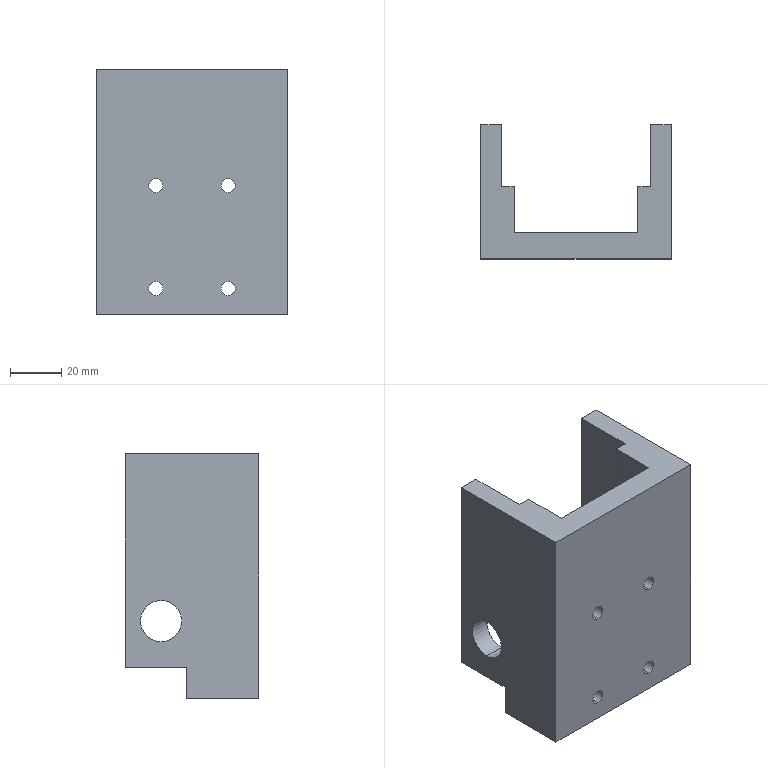Part | SolidWorks | features ICE 6, Extrusion 1 | 1 solid | 52 faces | box 74 x 52 x 95 mm | volume 141105 mm3 | cylinder 28 | plane 24 | commonest cylinder face diameters 5.5 x8 10 x8 2.5 x4 3 x4 16 x4
STEP:
#1=CARTESIAN_POINT('',(31.034,10.,22.));
#2=VERTEX_POINT('',#1);
#3=CARTESIAN_POINT('',(31.034,10.,38.));
#4=VERTEX_POINT('',#3);
#5=CARTESIAN_POINT('',(31.034,10.,30.));
#6=DIRECTION('',(-1.,0.,0.));
#7=DIRECTION('',(0.,0.,1.));
#8=AXIS2_PLACEMENT_3D('',#5,#6,#7);
#9=CIRCLE('',#8,8.);
#10=EDGE_CURVE('',#2,#4,#9,.T.);
#11=ORIENTED_EDGE('',*,*,#10,.F.);
#12=CARTESIAN_POINT('',(23.034,10.,22.));
#13=VERTEX_POINT('',#12);
#14=CARTESIAN_POINT('',(31.034,10.,22.));
#15=DIRECTION('',(-1.,0.,0.));
#16=VECTOR('',#15,1000.);
#17=LINE('',#14,#16);
#18=EDGE_CURVE('',#2,#13,#17,.T.);
#19=ORIENTED_EDGE('',*,*,#18,.T.);
#20=CARTESIAN_POINT('',(23.034,10.,38.));
#21=VERTEX_POINT('',#20);
#22=CARTESIAN_POINT('',(23.034,10.,30.));
#23=DIRECTION('',(1.,0.,0.));
#24=DIRECTION('',(0.,1.,0.));
#25=AXIS2_PLACEMENT_3D('',#22,#23,#24);
#26=CIRCLE('',#25,8.);
#27=EDGE_CURVE('',#21,#13,#26,.T.);
#28=ORIENTED_EDGE('',*,*,#27,.F.);
#29=CARTESIAN_POINT('',(31.034,10.,38.));
#30=DIRECTION('',(-1.,0.,0.));
#31=VECTOR('',#30,1000.);
#32=LINE('',#29,#31);
#33=EDGE_CURVE('',#4,#21,#32,.T.);
#34=ORIENTED_EDGE('',*,*,#33,.F.);
#35=EDGE_LOOP('',(#11,#19,#28,#34));
#36=FACE_OUTER_BOUND('',#35,.T.);
#37=CARTESIAN_POINT('',(31.034,10.,30.));
#38=DIRECTION('',(-1.,0.,0.));
#39=DIRECTION('',(0.,0.,1.));
#40=AXIS2_PLACEMENT_3D('',#37,#38,#39);
#41=CYLINDRICAL_SURFACE('',#40,8.);
#42=ADVANCED_FACE('',(#36),#41,.F.);
#43=CARTESIAN_POINT('',(-34.966,10.,22.));
#44=VERTEX_POINT('',#43);
#45=CARTESIAN_POINT('',(-34.966,10.,38.));
#46=VERTEX_POINT('',#45);
#47=CARTESIAN_POINT('',(-34.966,10.,30.));
#48=DIRECTION('',(-1.,0.,0.));
#49=DIRECTION('',(0.,0.,1.));
#50=AXIS2_PLACEMENT_3D('',#47,#48,#49);
#51=CIRCLE('',#50,8.);
#52=EDGE_CURVE('',#44,#46,#51,.T.);
#53=ORIENTED_EDGE('',*,*,#52,.F.);
#54=CARTESIAN_POINT('',(-42.966,10.,22.));
#55=VERTEX_POINT('',#54);
#56=CARTESIAN_POINT('',(31.034,10.,22.));
#57=DIRECTION('',(-1.,0.,0.));
#58=VECTOR('',#57,1000.);
#59=LINE('',#56,#58);
#60=EDGE_CURVE('',#44,#55,#59,.T.);
#61=ORIENTED_EDGE('',*,*,#60,.T.);
#62=CARTESIAN_POINT('',(-42.966,10.,38.));
#63=VERTEX_POINT('',#62);
#64=CARTESIAN_POINT('',(-42.966,10.,30.));
#65=DIRECTION('',(-1.,0.,0.));
#66=DIRECTION('',(0.,0.,1.));
#67=AXIS2_PLACEMENT_3D('',#64,#65,#66);
#68=CIRCLE('',#67,8.);
#69=EDGE_CURVE('',#55,#63,#68,.T.);
#70=ORIENTED_EDGE('',*,*,#69,.T.);
#71=CARTESIAN_POINT('',(31.034,10.,38.));
#72=DIRECTION('',(-1.,0.,0.));
#73=VECTOR('',#72,1000.);
#74=LINE('',#71,#73);
#75=EDGE_CURVE('',#46,#63,#74,.T.);
#76=ORIENTED_EDGE('',*,*,#75,.F.);
#77=EDGE_LOOP('',(#53,#61,#70,#76));
#78=FACE_OUTER_BOUND('',#77,.T.);
#79=CARTESIAN_POINT('',(31.034,10.,30.));
#80=DIRECTION('',(-1.,0.,0.));
#81=DIRECTION('',(0.,0.,1.));
#82=AXIS2_PLACEMENT_3D('',#79,#80,#81);
#83=CYLINDRICAL_SURFACE('',#82,8.);
#84=ADVANCED_FACE('',(#78),#83,.F.);
#85=CARTESIAN_POINT('',(-32.466,-7.5,8.75));
#86=VERTEX_POINT('',#85);
#87=CARTESIAN_POINT('',(-32.466,-7.5,11.25));
#88=VERTEX_POINT('',#87);
#89=CARTESIAN_POINT('',(-32.466,-7.5,10.));
#90=DIRECTION('',(0.,1.,0.));
#91=DIRECTION('',(0.,0.,1.));
#92=AXIS2_PLACEMENT_3D('',#89,#90,#91);
#93=CIRCLE('',#92,1.25);
#94=EDGE_CURVE('',#86,#88,#93,.T.);
#95=ORIENTED_EDGE('',*,*,#94,.F.);
#96=CARTESIAN_POINT('',(-32.466,-6.,8.75));
#97=VERTEX_POINT('',#96);
#98=CARTESIAN_POINT('',(-32.466,-7.5,8.75));
#99=DIRECTION('',(0.,1.,0.));
#100=VECTOR('',#99,1000.);
#101=LINE('',#98,#100);
#102=EDGE_CURVE('',#86,#97,#101,.T.);
#103=ORIENTED_EDGE('',*,*,#102,.T.);
#104=CARTESIAN_POINT('',(-32.466,-6.,11.25));
#105=VERTEX_POINT('',#104);
#106=CARTESIAN_POINT('',(-32.466,-6.,10.));
#107=DIRECTION('',(0.,-1.,0.));
#108=DIRECTION('',(0.,0.,1.));
#109=AXIS2_PLACEMENT_3D('',#106,#107,#108);
#110=CIRCLE('',#109,1.25);
#111=EDGE_CURVE('',#105,#97,#110,.T.);
#112=ORIENTED_EDGE('',*,*,#111,.F.);
#113=CARTESIAN_POINT('',(-32.466,-7.5,11.25));
#114=DIRECTION('',(0.,1.,0.));
#115=VECTOR('',#114,1000.);
#116=LINE('',#113,#115);
#117=EDGE_CURVE('',#88,#105,#116,.T.);
#118=ORIENTED_EDGE('',*,*,#117,.F.);
#119=EDGE_LOOP('',(#95,#103,#112,#118));
#120=FACE_OUTER_BOUND('',#119,.T.);
#121=CARTESIAN_POINT('',(-32.466,-7.5,10.));
#122=DIRECTION('',(0.,1.,0.));
#123=DIRECTION('',(0.,0.,1.));
#124=AXIS2_PLACEMENT_3D('',#121,#122,#123);
#125=CYLINDRICAL_SURFACE('',#124,1.25);
#126=ADVANCED_FACE('',(#120),#125,.F.);
#127=CARTESIAN_POINT('',(20.534,-7.5,8.75));
#128=VERTEX_POINT('',#127);
#129=CARTESIAN_POINT('',(20.534,-7.5,11.25));
#130=VERTEX_POINT('',#129);
#131=CARTESIAN_POINT('',(20.534,-7.5,10.));
#132=DIRECTION('',(0.,1.,0.));
#133=DIRECTION('',(0.,0.,1.));
#134=AXIS2_PLACEMENT_3D('',#131,#132,#133);
#135=CIRCLE('',#134,1.25);
#136=EDGE_CURVE('',#128,#130,#135,.T.);
#137=ORIENTED_EDGE('',*,*,#136,.F.);
#138=CARTESIAN_POINT('',(20.534,-6.,8.75));
#139=VERTEX_POINT('',#138);
#140=CARTESIAN_POINT('',(20.534,-7.5,8.75));
#141=DIRECTION('',(0.,1.,0.));
#142=VECTOR('',#141,1000.);
#143=LINE('',#140,#142);
#144=EDGE_CURVE('',#128,#139,#143,.T.);
#145=ORIENTED_EDGE('',*,*,#144,.T.);
#146=CARTESIAN_POINT('',(20.534,-6.,11.25));
#147=VERTEX_POINT('',#146);
#148=CARTESIAN_POINT('',(20.534,-6.,10.));
#149=DIRECTION('',(0.,-1.,0.));
#150=DIRECTION('',(0.,0.,1.));
#151=AXIS2_PLACEMENT_3D('',#148,#149,#150);
#152=CIRCLE('',#151,1.25);
#153=EDGE_CURVE('',#147,#139,#152,.T.);
#154=ORIENTED_EDGE('',*,*,#153,.F.);
#155=CARTESIAN_POINT('',(20.534,-7.5,11.25));
#156=DIRECTION('',(0.,1.,0.));
#157=VECTOR('',#156,1000.);
#158=LINE('',#155,#157);
#159=EDGE_CURVE('',#130,#147,#158,.T.);
#160=ORIENTED_EDGE('',*,*,#159,.F.);
#161=EDGE_LOOP('',(#137,#145,#154,#160));
#162=FACE_OUTER_BOUND('',#161,.T.);
#163=CARTESIAN_POINT('',(20.534,-7.5,10.));
#164=DIRECTION('',(0.,1.,0.));
#165=DIRECTION('',(0.,0.,1.));
#166=AXIS2_PLACEMENT_3D('',#163,#164,#165);
#167=CYLINDRICAL_SURFACE('',#166,1.25);
#168=ADVANCED_FACE('',(#162),#167,.F.);
#169=CARTESIAN_POINT('',(-32.466,-6.,8.5));
#170=VERTEX_POINT('',#169);
#171=CARTESIAN_POINT('',(-32.466,-6.,11.5));
#172=VERTEX_POINT('',#171);
#173=CARTESIAN_POINT('',(-32.466,-6.,10.));
#174=DIRECTION('',(0.,1.,0.));
#175=DIRECTION('',(0.,0.,1.));
#176=AXIS2_PLACEMENT_3D('',#173,#174,#175);
#177=CIRCLE('',#176,1.5);
#178=EDGE_CURVE('',#170,#172,#177,.T.);
#179=ORIENTED_EDGE('',*,*,#178,.F.);
#180=CARTESIAN_POINT('',(-32.466,0.,8.5));
#181=VERTEX_POINT('',#180);
#182=CARTESIAN_POINT('',(-32.466,-6.,8.5));
#183=DIRECTION('',(0.,1.,0.));
#184=VECTOR('',#183,1000.);
#185=LINE('',#182,#184);
#186=EDGE_CURVE('',#170,#181,#185,.T.);
#187=ORIENTED_EDGE('',*,*,#186,.T.);
#188=CARTESIAN_POINT('',(-32.466,0.,11.5));
#189=VERTEX_POINT('',#188);
#190=CARTESIAN_POINT('',(-32.466,0.,10.));
#191=DIRECTION('',(0.,1.,0.));
#192=DIRECTION('',(0.,0.,1.));
#193=AXIS2_PLACEMENT_3D('',#190,#191,#192);
#194=CIRCLE('',#193,1.5);
#195=EDGE_CURVE('',#181,#189,#194,.T.);
#196=ORIENTED_EDGE('',*,*,#195,.T.);
#197=CARTESIAN_POINT('',(-32.466,-6.,11.5));
#198=DIRECTION('',(0.,1.,0.));
#199=VECTOR('',#198,1000.);
#200=LINE('',#197,#199);
#201=EDGE_CURVE('',#172,#189,#200,.T.);
#202=ORIENTED_EDGE('',*,*,#201,.F.);
#203=EDGE_LOOP('',(#179,#187,#196,#202));
#204=FACE_OUTER_BOUND('',#203,.T.);
#205=CARTESIAN_POINT('',(-32.466,-6.,10.));
#206=DIRECTION('',(0.,1.,0.));
#207=DIRECTION('',(0.,0.,1.));
#208=AXIS2_PLACEMENT_3D('',#205,#206,#207);
#209=CYLINDRICAL_SURFACE('',#208,1.5);
#210=ADVANCED_FACE('',(#204),#209,.F.);
#211=CARTESIAN_POINT('',(20.534,-6.,8.5));
#212=VERTEX_POINT('',#211);
#213=CARTESIAN_POINT('',(20.534,-6.,11.5));
#214=VERTEX_POINT('',#213);
#215=CARTESIAN_POINT('',(20.534,-6.,10.));
#216=DIRECTION('',(0.,1.,0.));
#217=DIRECTION('',(0.,0.,1.));
#218=AXIS2_PLACEMENT_3D('',#215,#216,#217);
#219=CIRCLE('',#218,1.5);
#220=EDGE_CURVE('',#212,#214,#219,.T.);
#221=ORIENTED_EDGE('',*,*,#220,.F.);
#222=CARTESIAN_POINT('',(20.534,0.,8.5));
#223=VERTEX_POINT('',#222);
#224=CARTESIAN_POINT('',(20.534,-6.,8.5));
#225=DIRECTION('',(0.,1.,0.));
#226=VECTOR('',#225,1000.);
#227=LINE('',#224,#226);
#228=EDGE_CURVE('',#212,#223,#227,.T.);
#229=ORIENTED_EDGE('',*,*,#228,.T.);
#230=CARTESIAN_POINT('',(20.534,0.,11.5));
#231=VERTEX_POINT('',#230);
#232=CARTESIAN_POINT('',(20.534,0.,10.));
#233=DIRECTION('',(0.,1.,0.));
#234=DIRECTION('',(0.,0.,1.));
#235=AXIS2_PLACEMENT_3D('',#232,#233,#234);
#236=CIRCLE('',#235,1.5);
#237=EDGE_CURVE('',#223,#231,#236,.T.);
#238=ORIENTED_EDGE('',*,*,#237,.T.);
#239=CARTESIAN_POINT('',(20.534,-6.,11.5));
#240=DIRECTION('',(0.,1.,0.));
#241=VECTOR('',#240,1000.);
#242=LINE('',#239,#241);
#243=EDGE_CURVE('',#214,#231,#242,.T.);
#244=ORIENTED_EDGE('',*,*,#243,.F.);
#245=EDGE_LOOP('',(#221,#229,#238,#244));
#246=FACE_OUTER_BOUND('',#245,.T.);
#247=CARTESIAN_POINT('',(20.534,-6.,10.));
#248=DIRECTION('',(0.,1.,0.));
#249=DIRECTION('',(0.,0.,1.));
#250=AXIS2_PLACEMENT_3D('',#247,#248,#249);
#251=CYLINDRICAL_SURFACE('',#250,1.5);
#252=ADVANCED_FACE('',(#246),#251,.F.);
#253=CARTESIAN_POINT('',(-19.966,-23.75,5.));
#254=VERTEX_POINT('',#253);
#255=CARTESIAN_POINT('',(-19.966,-23.75,15.));
#256=VERTEX_POINT('',#255);
#257=CARTESIAN_POINT('',(-19.966,-23.75,10.));
#258=DIRECTION('',(0.,1.,0.));
#259=DIRECTION('',(0.,0.,1.));
#260=AXIS2_PLACEMENT_3D('',#257,#258,#259);
#261=CIRCLE('',#260,5.);
#262=EDGE_CURVE('',#254,#256,#261,.T.);
#263=ORIENTED_EDGE('',*,*,#262,.F.);
#264=CARTESIAN_POINT('',(-19.966,-18.,5.));
#265=VERTEX_POINT('',#264);
#266=CARTESIAN_POINT('',(-19.966,-23.75,5.));
#267=DIRECTION('',(0.,1.,0.));
#268=VECTOR('',#267,1000.);
#269=LINE('',#266,#268);
#270=EDGE_CURVE('',#254,#265,#269,.T.);
#271=ORIENTED_EDGE('',*,*,#270,.T.);
#272=CARTESIAN_POINT('',(-19.966,-18.,15.));
#273=VERTEX_POINT('',#272);
#274=CARTESIAN_POINT('',(-19.966,-18.,10.));
#275=DIRECTION('',(0.,1.,0.));
#276=DIRECTION('',(0.,0.,1.));
#277=AXIS2_PLACEMENT_3D('',#274,#275,#276);
#278=CIRCLE('',#277,5.);
#279=EDGE_CURVE('',#265,#273,#278,.T.);
#280=ORIENTED_EDGE('',*,*,#279,.T.);
#281=CARTESIAN_POINT('',(-19.966,-23.75,15.));
#282=DIRECTION('',(0.,1.,0.));
#283=VECTOR('',#282,1000.);
#284=LINE('',#281,#283);
#285=EDGE_CURVE('',#256,#273,#284,.T.);
#286=ORIENTED_EDGE('',*,*,#285,.F.);
#287=EDGE_LOOP('',(#263,#271,#280,#286));
#288=FACE_OUTER_BOUND('',#287,.T.);
#289=CARTESIAN_POINT('',(-19.966,-23.75,10.));
#290=DIRECTION('',(0.,1.,0.));
#291=DIRECTION('',(0.,0.,1.));
#292=AXIS2_PLACEMENT_3D('',#289,#290,#291);
#293=CYLINDRICAL_SURFACE('',#292,5.);
#294=ADVANCED_FACE('',(#288),#293,.F.);
#295=CARTESIAN_POINT('',(8.034,-23.75,45.));
#296=VERTEX_POINT('',#295);
#297=CARTESIAN_POINT('',(8.034,-23.75,55.));
#298=VERTEX_POINT('',#297);
#299=CARTESIAN_POINT('',(8.034,-23.75,50.));
#300=DIRECTION('',(0.,1.,0.));
#301=DIRECTION('',(0.,0.,1.));
#302=AXIS2_PLACEMENT_3D('',#299,#300,#301);
#303=CIRCLE('',#302,5.);
#304=EDGE_CURVE('',#296,#298,#303,.T.);
#305=ORIENTED_EDGE('',*,*,#304,.F.);
#306=CARTESIAN_POINT('',(8.034,-18.,45.));
#307=VERTEX_POINT('',#306);
#308=CARTESIAN_POINT('',(8.034,-23.75,45.));
#309=DIRECTION('',(0.,1.,0.));
#310=VECTOR('',#309,1000.);
#311=LINE('',#308,#310);
#312=EDGE_CURVE('',#296,#307,#311,.T.);
#313=ORIENTED_EDGE('',*,*,#312,.T.);
#314=CARTESIAN_POINT('',(8.034,-18.,55.));
#315=VERTEX_POINT('',#314);
#316=CARTESIAN_POINT('',(8.034,-18.,50.));
#317=DIRECTION('',(0.,1.,0.));
#318=DIRECTION('',(0.,0.,1.));
#319=AXIS2_PLACEMENT_3D('',#316,#317,#318);
#320=CIRCLE('',#319,5.);
#321=EDGE_CURVE('',#307,#315,#320,.T.);
#322=ORIENTED_EDGE('',*,*,#321,.T.);
#323=CARTESIAN_POINT('',(8.034,-23.75,55.));
#324=DIRECTION('',(0.,1.,0.));
#325=VECTOR('',#324,1000.);
#326=LINE('',#323,#325);
#327=EDGE_CURVE('',#298,#315,#326,.T.);
#328=ORIENTED_EDGE('',*,*,#327,.F.);
#329=EDGE_LOOP('',(#305,#313,#322,#328));
#330=FACE_OUTER_BOUND('',#329,.T.);
#331=CARTESIAN_POINT('',(8.034,-23.75,50.));
#332=DIRECTION('',(0.,1.,0.));
#333=DIRECTION('',(0.,0.,1.));
#334=AXIS2_PLACEMENT_3D('',#331,#332,#333);
#335=CYLINDRICAL_SURFACE('',#334,5.);
#336=ADVANCED_FACE('',(#330),#335,.F.);
#337=CARTESIAN_POINT('',(8.034,-23.75,5.));
#338=VERTEX_POINT('',#337);
#339=CARTESIAN_POINT('',(8.034,-23.75,15.));
#340=VERTEX_POINT('',#339);
#341=CARTESIAN_POINT('',(8.034,-23.75,10.));
#342=DIRECTION('',(0.,1.,0.));
#343=DIRECTION('',(0.,0.,1.));
#344=AXIS2_PLACEMENT_3D('',#341,#342,#343);
#345=CIRCLE('',#344,5.);
#346=EDGE_CURVE('',#338,#340,#345,.T.);
#347=ORIENTED_EDGE('',*,*,#346,.F.);
#348=CARTESIAN_POINT('',(8.034,-18.,5.));
#349=VERTEX_POINT('',#348);
#350=CARTESIAN_POINT('',(8.034,-23.75,5.));
#351=DIRECTION('',(0.,1.,0.));
#352=VECTOR('',#351,1000.);
#353=LINE('',#350,#352);
#354=EDGE_CURVE('',#338,#349,#353,.T.);
#355=ORIENTED_EDGE('',*,*,#354,.T.);
#356=CARTESIAN_POINT('',(8.034,-18.,15.));
#357=VERTEX_POINT('',#356);
#358=CARTESIAN_POINT('',(8.034,-18.,10.));
#359=DIRECTION('',(0.,1.,0.));
#360=DIRECTION('',(0.,0.,1.));
#361=AXIS2_PLACEMENT_3D('',#358,#359,#360);
#362=CIRCLE('',#361,5.);
#363=EDGE_CURVE('',#349,#357,#362,.T.);
#364=ORIENTED_EDGE('',*,*,#363,.T.);
#365=CARTESIAN_POINT('',(8.034,-23.75,15.));
#366=DIRECTION('',(0.,1.,0.));
#367=VECTOR('',#366,1000.);
#368=LINE('',#365,#367);
#369=EDGE_CURVE('',#340,#357,#368,.T.);
#370=ORIENTED_EDGE('',*,*,#369,.F.);
#371=EDGE_LOOP('',(#347,#355,#364,#370));
#372=FACE_OUTER_BOUND('',#371,.T.);
#373=CARTESIAN_POINT('',(8.034,-23.75,10.));
#374=DIRECTION('',(0.,1.,0.));
#375=DIRECTION('',(0.,0.,1.));
#376=AXIS2_PLACEMENT_3D('',#373,#374,#375);
#377=CYLINDRICAL_SURFACE('',#376,5.);
#378=ADVANCED_FACE('',(#372),#377,.F.);
#379=CARTESIAN_POINT('',(-19.966,-23.75,45.));
#380=VERTEX_POINT('',#379);
#381=CARTESIAN_POINT('',(-19.966,-23.75,55.));
#382=VERTEX_POINT('',#381);
#383=CARTESIAN_POINT('',(-19.966,-23.75,50.));
#384=DIRECTION('',(0.,1.,0.));
#385=DIRECTION('',(0.,0.,1.));
#386=AXIS2_PLACEMENT_3D('',#383,#384,#385);
#387=CIRCLE('',#386,5.);
#388=EDGE_CURVE('',#380,#382,#387,.T.);
#389=ORIENTED_EDGE('',*,*,#388,.F.);
#390=CARTESIAN_POINT('',(-19.966,-18.,45.));
#391=VERTEX_POINT('',#390);
#392=CARTESIAN_POINT('',(-19.966,-23.75,45.));
#393=DIRECTION('',(0.,1.,0.));
#394=VECTOR('',#393,1000.);
#395=LINE('',#392,#394);
#396=EDGE_CURVE('',#380,#391,#395,.T.);
#397=ORIENTED_EDGE('',*,*,#396,.T.);
#398=CARTESIAN_POINT('',(-19.966,-18.,55.));
#399=VERTEX_POINT('',#398);
#400=CARTESIAN_POINT('',(-19.966,-18.,50.));
#401=DIRECTION('',(0.,1.,0.));
#402=DIRECTION('',(0.,0.,1.));
#403=AXIS2_PLACEMENT_3D('',#400,#401,#402);
#404=CIRCLE('',#403,5.);
#405=EDGE_CURVE('',#391,#399,#404,.T.);
#406=ORIENTED_EDGE('',*,*,#405,.T.);
#407=CARTESIAN_POINT('',(-19.966,-23.75,55.));
#408=DIRECTION('',(0.,1.,0.));
#409=VECTOR('',#408,1000.);
#410=LINE('',#407,#409);
#411=EDGE_CURVE('',#382,#399,#410,.T.);
#412=ORIENTED_EDGE('',*,*,#411,.F.);
#413=EDGE_LOOP('',(#389,#397,#406,#412));
#414=FACE_OUTER_BOUND('',#413,.T.);
#415=CARTESIAN_POINT('',(-19.966,-23.75,50.));
#416=DIRECTION('',(0.,1.,0.));
#417=DIRECTION('',(0.,0.,1.));
#418=AXIS2_PLACEMENT_3D('',#415,#416,#417);
#419=CYLINDRICAL_SURFACE('',#418,5.);
#420=ADVANCED_FACE('',(#414),#419,.F.);
#421=CARTESIAN_POINT('',(-19.966,-28.,47.25));
#422=VERTEX_POINT('',#421);
#423=CARTESIAN_POINT('',(-19.966,-28.,52.75));
#424=VERTEX_POINT('',#423);
#425=CARTESIAN_POINT('',(-19.966,-28.,50.));
#426=DIRECTION('',(0.,1.,0.));
#427=DIRECTION('',(0.,0.,1.));
#428=AXIS2_PLACEMENT_3D('',#425,#426,#427);
#429=CIRCLE('',#428,2.75);
#430=EDGE_CURVE('',#422,#424,#429,.T.);
#431=ORIENTED_EDGE('',*,*,#430,.F.);
#432=CARTESIAN_POINT('',(-19.966,-23.75,47.25));
#433=VERTEX_POINT('',#432);
#434=CARTESIAN_POINT('',(-19.966,-28.,47.25));
#435=DIRECTION('',(0.,1.,0.));
#436=VECTOR('',#435,1000.);
#437=LINE('',#434,#436);
#438=EDGE_CURVE('',#422,#433,#437,.T.);
#439=ORIENTED_EDGE('',*,*,#438,.T.);
#440=CARTESIAN_POINT('',(-19.966,-23.75,52.75));
#441=VERTEX_POINT('',#440);
#442=CARTESIAN_POINT('',(-19.966,-23.75,50.));
#443=DIRECTION('',(0.,-1.,0.));
#444=DIRECTION('',(0.,0.,1.));
#445=AXIS2_PLACEMENT_3D('',#442,#443,#444);
#446=CIRCLE('',#445,2.75);
#447=EDGE_CURVE('',#441,#433,#446,.T.);
#448=ORIENTED_EDGE('',*,*,#447,.F.);
#449=CARTESIAN_POINT('',(-19.966,-28.,52.75));
#450=DIRECTION('',(0.,1.,0.));
#451=VECTOR('',#450,1000.);
#452=LINE('',#449,#451);
#453=EDGE_CURVE('',#424,#441,#452,.T.);
#454=ORIENTED_EDGE('',*,*,#453,.F.);
#455=EDGE_LOOP('',(#431,#439,#448,#454));
#456=FACE_OUTER_BOUND('',#455,.T.);
#457=CARTESIAN_POINT('',(-19.966,-28.,50.));
#458=DIRECTION('',(0.,1.,0.));
#459=DIRECTION('',(0.,0.,1.));
#460=AXIS2_PLACEMENT_3D('',#457,#458,#459);
#461=CYLINDRICAL_SURFACE('',#460,2.75);
#462=ADVANCED_FACE('',(#456),#461,.F.);
#463=CARTESIAN_POINT('',(8.034,-28.,7.25));
#464=VERTEX_POINT('',#463);
#465=CARTESIAN_POINT('',(8.034,-28.,12.75));
#466=VERTEX_POINT('',#465);
#467=CARTESIAN_POINT('',(8.034,-28.,10.));
#468=DIRECTION('',(0.,1.,0.));
#469=DIRECTION('',(0.,0.,1.));
#470=AXIS2_PLACEMENT_3D('',#467,#468,#469);
#471=CIRCLE('',#470,2.75);
#472=EDGE_CURVE('',#464,#466,#471,.T.);
#473=ORIENTED_EDGE('',*,*,#472,.F.);
#474=CARTESIAN_POINT('',(8.034,-23.75,7.25));
#475=VERTEX_POINT('',#474);
#476=CARTESIAN_POINT('',(8.034,-28.,7.25));
#477=DIRECTION('',(0.,1.,0.));
#478=VECTOR('',#477,1000.);
#479=LINE('',#476,#478);
#480=EDGE_CURVE('',#464,#475,#479,.T.);
#481=ORIENTED_EDGE('',*,*,#480,.T.);
#482=CARTESIAN_POINT('',(8.034,-23.75,12.75));
#483=VERTEX_POINT('',#482);
#484=CARTESIAN_POINT('',(8.034,-23.75,10.));
#485=DIRECTION('',(0.,-1.,0.));
#486=DIRECTION('',(0.,0.,1.));
#487=AXIS2_PLACEMENT_3D('',#484,#485,#486);
#488=CIRCLE('',#487,2.75);
#489=EDGE_CURVE('',#483,#475,#488,.T.);
#490=ORIENTED_EDGE('',*,*,#489,.F.);
#491=CARTESIAN_POINT('',(8.034,-28.,12.75));
#492=DIRECTION('',(0.,1.,0.));
#493=VECTOR('',#492,1000.);
#494=LINE('',#491,#493);
#495=EDGE_CURVE('',#466,#483,#494,.T.);
#496=ORIENTED_EDGE('',*,*,#495,.F.);
#497=EDGE_LOOP('',(#473,#481,#490,#496));
#498=FACE_OUTER_BOUND('',#497,.T.);
#499=CARTESIAN_POINT('',(8.034,-28.,10.));
#500=DIRECTION('',(0.,1.,0.));
#501=DIRECTION('',(0.,0.,1.));
#502=AXIS2_PLACEMENT_3D('',#499,#500,#501);
#503=CYLINDRICAL_SURFACE('',#502,2.75);
#504=ADVANCED_FACE('',(#498),#503,.F.);
#505=CARTESIAN_POINT('',(8.034,-28.,47.25));
#506=VERTEX_POINT('',#505);
#507=CARTESIAN_POINT('',(8.034,-28.,52.75));
#508=VERTEX_POINT('',#507);
#509=CARTESIAN_POINT('',(8.034,-28.,50.));
#510=DIRECTION('',(0.,1.,0.));
#511=DIRECTION('',(0.,0.,1.));
#512=AXIS2_PLACEMENT_3D('',#509,#510,#511);
#513=CIRCLE('',#512,2.75);
#514=EDGE_CURVE('',#506,#508,#513,.T.);
#515=ORIENTED_EDGE('',*,*,#514,.F.);
#516=CARTESIAN_POINT('',(8.034,-23.75,47.25));
#517=VERTEX_POINT('',#516);
#518=CARTESIAN_POINT('',(8.034,-28.,47.25));
#519=DIRECTION('',(0.,1.,0.));
#520=VECTOR('',#519,1000.);
#521=LINE('',#518,#520);
#522=EDGE_CURVE('',#506,#517,#521,.T.);
#523=ORIENTED_EDGE('',*,*,#522,.T.);
#524=CARTESIAN_POINT('',(8.034,-23.75,52.75));
#525=VERTEX_POINT('',#524);
#526=CARTESIAN_POINT('',(8.034,-23.75,50.));
#527=DIRECTION('',(0.,-1.,0.));
#528=DIRECTION('',(0.,0.,1.));
#529=AXIS2_PLACEMENT_3D('',#526,#527,#528);
#530=CIRCLE('',#529,2.75);
#531=EDGE_CURVE('',#525,#517,#530,.T.);
#532=ORIENTED_EDGE('',*,*,#531,.F.);
#533=CARTESIAN_POINT('',(8.034,-28.,52.75));
#534=DIRECTION('',(0.,1.,0.));
#535=VECTOR('',#534,1000.);
#536=LINE('',#533,#535);
#537=EDGE_CURVE('',#508,#525,#536,.T.);
#538=ORIENTED_EDGE('',*,*,#537,.F.);
#539=EDGE_LOOP('',(#515,#523,#532,#538));
#540=FACE_OUTER_BOUND('',#539,.T.);
#541=CARTESIAN_POINT('',(8.034,-28.,50.));
#542=DIRECTION('',(0.,1.,0.));
#543=DIRECTION('',(0.,0.,1.));
#544=AXIS2_PLACEMENT_3D('',#541,#542,#543);
#545=CYLINDRICAL_SURFACE('',#544,2.75);
#546=ADVANCED_FACE('',(#540),#545,.F.);
#547=CARTESIAN_POINT('',(-19.966,-28.,7.25));
#548=VERTEX_POINT('',#547);
#549=CARTESIAN_POINT('',(-19.966,-28.,12.75));
#550=VERTEX_POINT('',#549);
#551=CARTESIAN_POINT('',(-19.966,-28.,10.));
#552=DIRECTION('',(0.,1.,0.));
#553=DIRECTION('',(0.,0.,1.));
#554=AXIS2_PLACEMENT_3D('',#551,#552,#553);
#555=CIRCLE('',#554,2.75);
#556=EDGE_CURVE('',#548,#550,#555,.T.);
#557=ORIENTED_EDGE('',*,*,#556,.F.);
#558=CARTESIAN_POINT('',(-19.966,-23.75,7.25));
#559=VERTEX_POINT('',#558);
#560=CARTESIAN_POINT('',(-19.966,-28.,7.25));
#561=DIRECTION('',(0.,1.,0.));
#562=VECTOR('',#561,1000.);
#563=LINE('',#560,#562);
#564=EDGE_CURVE('',#548,#559,#563,.T.);
#565=ORIENTED_EDGE('',*,*,#564,.T.);
#566=CARTESIAN_POINT('',(-19.966,-23.75,12.75));
#567=VERTEX_POINT('',#566);
#568=CARTESIAN_POINT('',(-19.966,-23.75,10.));
#569=DIRECTION('',(0.,-1.,0.));
#570=DIRECTION('',(0.,0.,1.));
#571=AXIS2_PLACEMENT_3D('',#568,#569,#570);
#572=CIRCLE('',#571,2.75);
#573=EDGE_CURVE('',#567,#559,#572,.T.);
#574=ORIENTED_EDGE('',*,*,#573,.F.);
#575=CARTESIAN_POINT('',(-19.966,-28.,12.75));
#576=DIRECTION('',(0.,1.,0.));
#577=VECTOR('',#576,1000.);
#578=LINE('',#575,#577);
#579=EDGE_CURVE('',#550,#567,#578,.T.);
#580=ORIENTED_EDGE('',*,*,#579,.F.);
#581=EDGE_LOOP('',(#557,#565,#574,#580));
#582=FACE_OUTER_BOUND('',#581,.T.);
#583=CARTESIAN_POINT('',(-19.966,-28.,10.));
#584=DIRECTION('',(0.,1.,0.));
#585=DIRECTION('',(0.,0.,1.));
#586=AXIS2_PLACEMENT_3D('',#583,#584,#585);
#587=CYLINDRICAL_SURFACE('',#586,2.75);
#588=ADVANCED_FACE('',(#582),#587,.F.);
#589=ORIENTED_EDGE('',*,*,#564,.F.);
#590=CARTESIAN_POINT('',(-19.966,-28.,10.));
#591=DIRECTION('',(0.,1.,0.));
#592=DIRECTION('',(0.,0.,1.));
#593=AXIS2_PLACEMENT_3D('',#590,#591,#592);
#594=CIRCLE('',#593,2.75);
#595=EDGE_CURVE('',#550,#548,#594,.T.);
#596=ORIENTED_EDGE('',*,*,#595,.F.);
#597=ORIENTED_EDGE('',*,*,#579,.T.);
#598=CARTESIAN_POINT('',(-19.966,-23.75,10.));
#599=DIRECTION('',(0.,-1.,0.));
#600=DIRECTION('',(0.,0.,1.));
#601=AXIS2_PLACEMENT_3D('',#598,#599,#600);
#602=CIRCLE('',#601,2.75);
#603=EDGE_CURVE('',#559,#567,#602,.T.);
#604=ORIENTED_EDGE('',*,*,#603,.F.);
#605=EDGE_LOOP('',(#589,#596,#597,#604));
#606=FACE_OUTER_BOUND('',#605,.T.);
#607=CARTESIAN_POINT('',(-19.966,-28.,10.));
#608=DIRECTION('',(0.,1.,0.));
#609=DIRECTION('',(0.,0.,1.));
#610=AXIS2_PLACEMENT_3D('',#607,#608,#609);
#611=CYLINDRICAL_SURFACE('',#610,2.75);
#612=ADVANCED_FACE('',(#606),#611,.F.);
#613=ORIENTED_EDGE('',*,*,#522,.F.);
#614=CARTESIAN_POINT('',(8.034,-28.,50.));
#615=DIRECTION('',(0.,1.,0.));
#616=DIRECTION('',(0.,0.,1.));
#617=AXIS2_PLACEMENT_3D('',#614,#615,#616);
#618=CIRCLE('',#617,2.75);
#619=EDGE_CURVE('',#508,#506,#618,.T.);
#620=ORIENTED_EDGE('',*,*,#619,.F.);
#621=ORIENTED_EDGE('',*,*,#537,.T.);
#622=CARTESIAN_POINT('',(8.034,-23.75,50.));
#623=DIRECTION('',(0.,-1.,0.));
#624=DIRECTION('',(0.,0.,1.));
#625=AXIS2_PLACEMENT_3D('',#622,#623,#624);
#626=CIRCLE('',#625,2.75);
#627=EDGE_CURVE('',#517,#525,#626,.T.);
#628=ORIENTED_EDGE('',*,*,#627,.F.);
#629=EDGE_LOOP('',(#613,#620,#621,#628));
#630=FACE_OUTER_BOUND('',#629,.T.);
#631=CARTESIAN_POINT('',(8.034,-28.,50.));
#632=DIRECTION('',(0.,1.,0.));
#633=DIRECTION('',(0.,0.,1.));
#634=AXIS2_PLACEMENT_3D('',#631,#632,#633);
#635=CYLINDRICAL_SURFACE('',#634,2.75);
#636=ADVANCED_FACE('',(#630),#635,.F.);
#637=ORIENTED_EDGE('',*,*,#480,.F.);
#638=CARTESIAN_POINT('',(8.034,-28.,10.));
#639=DIRECTION('',(0.,1.,0.));
#640=DIRECTION('',(0.,0.,1.));
#641=AXIS2_PLACEMENT_3D('',#638,#639,#640);
#642=CIRCLE('',#641,2.75);
#643=EDGE_CURVE('',#466,#464,#642,.T.);
#644=ORIENTED_EDGE('',*,*,#643,.F.);
#645=ORIENTED_EDGE('',*,*,#495,.T.);
#646=CARTESIAN_POINT('',(8.034,-23.75,10.));
#647=DIRECTION('',(0.,-1.,0.));
#648=DIRECTION('',(0.,0.,1.));
#649=AXIS2_PLACEMENT_3D('',#646,#647,#648);
#650=CIRCLE('',#649,2.75);
#651=EDGE_CURVE('',#475,#483,#650,.T.);
#652=ORIENTED_EDGE('',*,*,#651,.F.);
#653=EDGE_LOOP('',(#637,#644,#645,#652));
#654=FACE_OUTER_BOUND('',#653,.T.);
#655=CARTESIAN_POINT('',(8.034,-28.,10.));
#656=DIRECTION('',(0.,1.,0.));
#657=DIRECTION('',(0.,0.,1.));
#658=AXIS2_PLACEMENT_3D('',#655,#656,#657);
#659=CYLINDRICAL_SURFACE('',#658,2.75);
#660=ADVANCED_FACE('',(#654),#659,.F.);
#661=ORIENTED_EDGE('',*,*,#438,.F.);
#662=CARTESIAN_POINT('',(-19.966,-28.,50.));
#663=DIRECTION('',(0.,1.,0.));
#664=DIRECTION('',(0.,0.,1.));
#665=AXIS2_PLACEMENT_3D('',#662,#663,#664);
#666=CIRCLE('',#665,2.75);
#667=EDGE_CURVE('',#424,#422,#666,.T.);
#668=ORIENTED_EDGE('',*,*,#667,.F.);
#669=ORIENTED_EDGE('',*,*,#453,.T.);
#670=CARTESIAN_POINT('',(-19.966,-23.75,50.));
#671=DIRECTION('',(0.,-1.,0.));
#672=DIRECTION('',(0.,0.,1.));
#673=AXIS2_PLACEMENT_3D('',#670,#671,#672);
#674=CIRCLE('',#673,2.75);
#675=EDGE_CURVE('',#433,#441,#674,.T.);
#676=ORIENTED_EDGE('',*,*,#675,.F.);
#677=EDGE_LOOP('',(#661,#668,#669,#676));
#678=FACE_OUTER_BOUND('',#677,.T.);
#679=CARTESIAN_POINT('',(-19.966,-28.,50.));
#680=DIRECTION('',(0.,1.,0.));
#681=DIRECTION('',(0.,0.,1.));
#682=AXIS2_PLACEMENT_3D('',#679,#680,#681);
#683=CYLINDRICAL_SURFACE('',#682,2.75);
#684=ADVANCED_FACE('',(#678),#683,.F.);
#685=CARTESIAN_POINT('',(-34.966,24.,95.));
#686=VERTEX_POINT('',#685);
#687=CARTESIAN_POINT('',(-34.966,24.,12.));
#688=VERTEX_POINT('',#687);
#689=CARTESIAN_POINT('',(-34.966,24.,95.));
#690=DIRECTION('',(0.,0.,-1.));
#691=VECTOR('',#690,1000.);
#692=LINE('',#689,#691);
#693=EDGE_CURVE('',#686,#688,#692,.T.);
#694=ORIENTED_EDGE('',*,*,#693,.T.);
#695=CARTESIAN_POINT('',(-42.966,24.,12.));
#696=VERTEX_POINT('',#695);
#697=CARTESIAN_POINT('',(31.034,24.,12.));
#698=DIRECTION('',(-1.,0.,0.));
#699=VECTOR('',#698,1000.);
#700=LINE('',#697,#699);
#701=EDGE_CURVE('',#688,#696,#700,.T.);
#702=ORIENTED_EDGE('',*,*,#701,.T.);
#703=CARTESIAN_POINT('',(-42.966,24.,95.));
#704=VERTEX_POINT('',#703);
#705=CARTESIAN_POINT('',(-42.966,24.,95.));
#706=DIRECTION('',(0.,0.,-1.));
#707=VECTOR('',#706,1000.);
#708=LINE('',#705,#707);
#709=EDGE_CURVE('',#704,#696,#708,.T.);
#710=ORIENTED_EDGE('',*,*,#709,.F.);
#711=CARTESIAN_POINT('',(-42.966,24.,95.));
#712=DIRECTION('',(-1.,0.,0.));
#713=VECTOR('',#712,1000.);
#714=LINE('',#711,#713);
#715=EDGE_CURVE('',#686,#704,#714,.T.);
#716=ORIENTED_EDGE('',*,*,#715,.F.);
#717=EDGE_LOOP('',(#694,#702,#710,#716));
#718=FACE_OUTER_BOUND('',#717,.T.);
#719=CARTESIAN_POINT('',(-42.966,24.,95.));
#720=DIRECTION('',(0.,-1.,0.));
#721=DIRECTION('',(0.,0.,-1.));
#722=AXIS2_PLACEMENT_3D('',#719,#720,#721);
#723=PLANE('',#722);
#724=ADVANCED_FACE('',(#718),#723,.F.);
#725=CARTESIAN_POINT('',(-42.966,10.,30.));
#726=DIRECTION('',(-1.,0.,0.));
#727=DIRECTION('',(0.,0.,1.));
#728=AXIS2_PLACEMENT_3D('',#725,#726,#727);
#729=CIRCLE('',#728,8.);
#730=EDGE_CURVE('',#63,#55,#729,.T.);
#731=ORIENTED_EDGE('',*,*,#730,.F.);
#732=ORIENTED_EDGE('',*,*,#69,.F.);
#733=EDGE_LOOP('',(#731,#732));
#734=FACE_BOUND('',#733,.T.);
#735=ORIENTED_EDGE('',*,*,#709,.T.);
#736=CARTESIAN_POINT('',(-42.966,0.,12.));
#737=VERTEX_POINT('',#736);
#738=CARTESIAN_POINT('',(-42.966,0.,12.));
#739=DIRECTION('',(0.,1.,0.));
#740=VECTOR('',#739,1000.);
#741=LINE('',#738,#740);
#742=EDGE_CURVE('',#737,#696,#741,.T.);
#743=ORIENTED_EDGE('',*,*,#742,.F.);
#744=CARTESIAN_POINT('',(-42.966,0.,0.));
#745=VERTEX_POINT('',#744);
#746=CARTESIAN_POINT('',(-42.966,0.,0.));
#747=DIRECTION('',(0.,0.,1.));
#748=VECTOR('',#747,1000.);
#749=LINE('',#746,#748);
#750=EDGE_CURVE('',#745,#737,#749,.T.);
#751=ORIENTED_EDGE('',*,*,#750,.F.);
#752=CARTESIAN_POINT('',(-42.966,-28.,0.));
#753=VERTEX_POINT('',#752);
#754=CARTESIAN_POINT('',(-42.966,24.,0.));
#755=DIRECTION('',(0.,-1.,0.));
#756=VECTOR('',#755,1000.);
#757=LINE('',#754,#756);
#758=EDGE_CURVE('',#745,#753,#757,.T.);
#759=ORIENTED_EDGE('',*,*,#758,.T.);
#760=CARTESIAN_POINT('',(-42.966,-28.,95.));
#761=VERTEX_POINT('',#760);
#762=CARTESIAN_POINT('',(-42.966,-28.,95.));
#763=DIRECTION('',(0.,0.,-1.));
#764=VECTOR('',#763,1000.);
#765=LINE('',#762,#764);
#766=EDGE_CURVE('',#761,#753,#765,.T.);
#767=ORIENTED_EDGE('',*,*,#766,.F.);
#768=CARTESIAN_POINT('',(-42.966,24.,95.));
#769=DIRECTION('',(0.,-1.,0.));
#770=VECTOR('',#769,1000.);
#771=LINE('',#768,#770);
#772=EDGE_CURVE('',#704,#761,#771,.T.);
#773=ORIENTED_EDGE('',*,*,#772,.F.);
#774=EDGE_LOOP('',(#735,#743,#751,#759,#767,#773));
#775=FACE_OUTER_BOUND('',#774,.T.);
#776=CARTESIAN_POINT('',(-42.966,24.,95.));
#777=DIRECTION('',(1.,0.,0.));
#778=DIRECTION('',(0.,0.,-1.));
#779=AXIS2_PLACEMENT_3D('',#776,#777,#778);
#780=PLANE('',#779);
#781=ADVANCED_FACE('',(#734,#775),#780,.F.);
#782=ORIENTED_EDGE('',*,*,#667,.T.);
#783=ORIENTED_EDGE('',*,*,#430,.T.);
#784=EDGE_LOOP('',(#782,#783));
#785=FACE_BOUND('',#784,.T.);
#786=ORIENTED_EDGE('',*,*,#643,.T.);
#787=ORIENTED_EDGE('',*,*,#472,.T.);
#788=EDGE_LOOP('',(#786,#787));
#789=FACE_BOUND('',#788,.T.);
#790=ORIENTED_EDGE('',*,*,#619,.T.);
#791=ORIENTED_EDGE('',*,*,#514,.T.);
#792=EDGE_LOOP('',(#790,#791));
#793=FACE_BOUND('',#792,.T.);
#794=ORIENTED_EDGE('',*,*,#595,.T.);
#795=ORIENTED_EDGE('',*,*,#556,.T.);
#796=EDGE_LOOP('',(#794,#795));
#797=FACE_BOUND('',#796,.T.);
#798=CARTESIAN_POINT('',(31.034,-28.,0.));
#799=VERTEX_POINT('',#798);
#800=CARTESIAN_POINT('',(-42.966,-28.,0.));
#801=DIRECTION('',(1.,0.,0.));
#802=VECTOR('',#801,1000.);
#803=LINE('',#800,#802);
#804=EDGE_CURVE('',#753,#799,#803,.T.);
#805=ORIENTED_EDGE('',*,*,#804,.T.);
#806=CARTESIAN_POINT('',(31.034,-28.,95.));
#807=VERTEX_POINT('',#806);
#808=CARTESIAN_POINT('',(31.034,-28.,95.));
#809=DIRECTION('',(0.,0.,-1.));
#810=VECTOR('',#809,1000.);
#811=LINE('',#808,#810);
#812=EDGE_CURVE('',#807,#799,#811,.T.);
#813=ORIENTED_EDGE('',*,*,#812,.F.);
#814=CARTESIAN_POINT('',(-42.966,-28.,95.));
#815=DIRECTION('',(1.,0.,0.));
#816=VECTOR('',#815,1000.);
#817=LINE('',#814,#816);
#818=EDGE_CURVE('',#761,#807,#817,.T.);
#819=ORIENTED_EDGE('',*,*,#818,.F.);
#820=ORIENTED_EDGE('',*,*,#766,.T.);
#821=EDGE_LOOP('',(#805,#813,#819,#820));
#822=FACE_OUTER_BOUND('',#821,.T.);
#823=CARTESIAN_POINT('',(-42.966,-28.,95.));
#824=DIRECTION('',(0.,1.,0.));
#825=DIRECTION('',(0.,0.,1.));
#826=AXIS2_PLACEMENT_3D('',#823,#824,#825);
#827=PLANE('',#826);
#828=ADVANCED_FACE('',(#785,#789,#793,#797,#822),#827,.F.);
#829=CARTESIAN_POINT('',(31.034,10.,30.));
#830=DIRECTION('',(-1.,0.,0.));
#831=DIRECTION('',(0.,0.,1.));
#832=AXIS2_PLACEMENT_3D('',#829,#830,#831);
#833=CIRCLE('',#832,8.);
#834=EDGE_CURVE('',#4,#2,#833,.T.);
#835=ORIENTED_EDGE('',*,*,#834,.T.);
#836=ORIENTED_EDGE('',*,*,#10,.T.);
#837=EDGE_LOOP('',(#835,#836));
#838=FACE_BOUND('',#837,.T.);
#839=CARTESIAN_POINT('',(31.034,0.,0.));
#840=VERTEX_POINT('',#839);
#841=CARTESIAN_POINT('',(31.034,0.,12.));
#842=VERTEX_POINT('',#841);
#843=CARTESIAN_POINT('',(31.034,0.,0.));
#844=DIRECTION('',(0.,0.,1.));
#845=VECTOR('',#844,1000.);
#846=LINE('',#843,#845);
#847=EDGE_CURVE('',#840,#842,#846,.T.);
#848=ORIENTED_EDGE('',*,*,#847,.T.);
#849=CARTESIAN_POINT('',(31.034,24.,12.));
#850=VERTEX_POINT('',#849);
#851=CARTESIAN_POINT('',(31.034,0.,12.));
#852=DIRECTION('',(0.,1.,0.));
#853=VECTOR('',#852,1000.);
#854=LINE('',#851,#853);
#855=EDGE_CURVE('',#842,#850,#854,.T.);
#856=ORIENTED_EDGE('',*,*,#855,.T.);
#857=CARTESIAN_POINT('',(31.034,24.,95.));
#858=VERTEX_POINT('',#857);
#859=CARTESIAN_POINT('',(31.034,24.,95.));
#860=DIRECTION('',(0.,0.,-1.));
#861=VECTOR('',#860,1000.);
#862=LINE('',#859,#861);
#863=EDGE_CURVE('',#858,#850,#862,.T.);
#864=ORIENTED_EDGE('',*,*,#863,.F.);
#865=CARTESIAN_POINT('',(31.034,-28.,95.));
#866=DIRECTION('',(0.,1.,0.));
#867=VECTOR('',#866,1000.);
#868=LINE('',#865,#867);
#869=EDGE_CURVE('',#807,#858,#868,.T.);
#870=ORIENTED_EDGE('',*,*,#869,.F.);
#871=ORIENTED_EDGE('',*,*,#812,.T.);
#872=CARTESIAN_POINT('',(31.034,-28.,0.));
#873=DIRECTION('',(0.,1.,0.));
#874=VECTOR('',#873,1000.);
#875=LINE('',#872,#874);
#876=EDGE_CURVE('',#799,#840,#875,.T.);
#877=ORIENTED_EDGE('',*,*,#876,.T.);
#878=EDGE_LOOP('',(#848,#856,#864,#870,#871,#877));
#879=FACE_OUTER_BOUND('',#878,.T.);
#880=CARTESIAN_POINT('',(31.034,-28.,95.));
#881=DIRECTION('',(-1.,0.,0.));
#882=DIRECTION('',(0.,-1.,0.));
#883=AXIS2_PLACEMENT_3D('',#880,#881,#882);
#884=PLANE('',#883);
#885=ADVANCED_FACE('',(#838,#879),#884,.F.);
#886=ORIENTED_EDGE('',*,*,#863,.T.);
#887=CARTESIAN_POINT('',(23.034,24.,12.));
#888=VERTEX_POINT('',#887);
#889=CARTESIAN_POINT('',(31.034,24.,12.));
#890=DIRECTION('',(-1.,0.,0.));
#891=VECTOR('',#890,1000.);
#892=LINE('',#889,#891);
#893=EDGE_CURVE('',#850,#888,#892,.T.);
#894=ORIENTED_EDGE('',*,*,#893,.T.);
#895=CARTESIAN_POINT('',(23.034,24.,95.));
#896=VERTEX_POINT('',#895);
#897=CARTESIAN_POINT('',(23.034,24.,95.));
#898=DIRECTION('',(0.,0.,-1.));
#899=VECTOR('',#898,1000.);
#900=LINE('',#897,#899);
#901=EDGE_CURVE('',#896,#888,#900,.T.);
#902=ORIENTED_EDGE('',*,*,#901,.F.);
#903=CARTESIAN_POINT('',(23.034,24.,95.));
#904=DIRECTION('',(-1.,0.,0.));
#905=VECTOR('',#904,1000.);
#906=LINE('',#903,#905);
#907=EDGE_CURVE('',#858,#896,#906,.T.);
#908=ORIENTED_EDGE('',*,*,#907,.F.);
#909=EDGE_LOOP('',(#886,#894,#902,#908));
#910=FACE_OUTER_BOUND('',#909,.T.);
#911=CARTESIAN_POINT('',(23.034,24.,95.));
#912=DIRECTION('',(0.,-1.,0.));
#913=DIRECTION('',(0.,0.,-1.));
#914=AXIS2_PLACEMENT_3D('',#911,#912,#913);
#915=PLANE('',#914);
#916=ADVANCED_FACE('',(#910),#915,.F.);
#917=ORIENTED_EDGE('',*,*,#27,.T.);
#918=CARTESIAN_POINT('',(23.034,10.,30.));
#919=DIRECTION('',(1.,0.,0.));
#920=DIRECTION('',(0.,1.,0.));
#921=AXIS2_PLACEMENT_3D('',#918,#919,#920);
#922=CIRCLE('',#921,8.);
#923=EDGE_CURVE('',#13,#21,#922,.T.);
#924=ORIENTED_EDGE('',*,*,#923,.T.);
#925=EDGE_LOOP('',(#917,#924));
#926=FACE_BOUND('',#925,.T.);
#927=ORIENTED_EDGE('',*,*,#901,.T.);
#928=CARTESIAN_POINT('',(23.034,0.,12.));
#929=VERTEX_POINT('',#928);
#930=CARTESIAN_POINT('',(23.034,0.,12.));
#931=DIRECTION('',(0.,-1.,0.));
#932=VECTOR('',#931,1000.);
#933=LINE('',#930,#932);
#934=EDGE_CURVE('',#888,#929,#933,.T.);
#935=ORIENTED_EDGE('',*,*,#934,.T.);
#936=CARTESIAN_POINT('',(23.034,0.,95.));
#937=VERTEX_POINT('',#936);
#938=CARTESIAN_POINT('',(23.034,0.,95.));
#939=DIRECTION('',(0.,0.,-1.));
#940=VECTOR('',#939,1000.);
#941=LINE('',#938,#940);
#942=EDGE_CURVE('',#937,#929,#941,.T.);
#943=ORIENTED_EDGE('',*,*,#942,.F.);
#944=CARTESIAN_POINT('',(23.034,0.,95.));
#945=DIRECTION('',(0.,-1.,0.));
#946=VECTOR('',#945,1000.);
#947=LINE('',#944,#946);
#948=EDGE_CURVE('',#896,#937,#947,.T.);
#949=ORIENTED_EDGE('',*,*,#948,.F.);
#950=EDGE_LOOP('',(#927,#935,#943,#949));
#951=FACE_OUTER_BOUND('',#950,.T.);
#952=CARTESIAN_POINT('',(23.034,0.,95.));
#953=DIRECTION('',(1.,0.,0.));
#954=DIRECTION('',(0.,1.,0.));
#955=AXIS2_PLACEMENT_3D('',#952,#953,#954);
#956=PLANE('',#955);
#957=ADVANCED_FACE('',(#926,#951),#956,.F.);
#958=CARTESIAN_POINT('',(20.534,0.,10.));
#959=DIRECTION('',(0.,1.,0.));
#960=DIRECTION('',(0.,0.,1.));
#961=AXIS2_PLACEMENT_3D('',#958,#959,#960);
#962=CIRCLE('',#961,1.5);
#963=EDGE_CURVE('',#231,#223,#962,.T.);
#964=ORIENTED_EDGE('',*,*,#963,.F.);
#965=ORIENTED_EDGE('',*,*,#237,.F.);
#966=EDGE_LOOP('',(#964,#965));
#967=FACE_BOUND('',#966,.T.);
#968=ORIENTED_EDGE('',*,*,#942,.T.);
#969=CARTESIAN_POINT('',(31.034,0.,12.));
#970=DIRECTION('',(-1.,0.,0.));
#971=VECTOR('',#970,1000.);
#972=LINE('',#969,#971);
#973=EDGE_CURVE('',#842,#929,#972,.T.);
#974=ORIENTED_EDGE('',*,*,#973,.F.);
#975=ORIENTED_EDGE('',*,*,#847,.F.);
#976=CARTESIAN_POINT('',(18.034,0.,0.));
#977=VERTEX_POINT('',#976);
#978=CARTESIAN_POINT('',(18.034,0.,0.));
#979=DIRECTION('',(-1.,0.,0.));
#980=VECTOR('',#979,1000.);
#981=LINE('',#978,#980);
#982=EDGE_CURVE('',#840,#977,#981,.T.);
#983=ORIENTED_EDGE('',*,*,#982,.T.);
#984=CARTESIAN_POINT('',(18.034,0.,95.));
#985=VERTEX_POINT('',#984);
#986=CARTESIAN_POINT('',(18.034,0.,95.));
#987=DIRECTION('',(0.,0.,-1.));
#988=VECTOR('',#987,1000.);
#989=LINE('',#986,#988);
#990=EDGE_CURVE('',#985,#977,#989,.T.);
#991=ORIENTED_EDGE('',*,*,#990,.F.);
#992=CARTESIAN_POINT('',(18.034,0.,95.));
#993=DIRECTION('',(-1.,0.,0.));
#994=VECTOR('',#993,1000.);
#995=LINE('',#992,#994);
#996=EDGE_CURVE('',#937,#985,#995,.T.);
#997=ORIENTED_EDGE('',*,*,#996,.F.);
#998=EDGE_LOOP('',(#968,#974,#975,#983,#991,#997));
#999=FACE_OUTER_BOUND('',#998,.T.);
#1000=CARTESIAN_POINT('',(18.034,0.,95.));
#1001=DIRECTION('',(0.,-1.,0.));
#1002=DIRECTION('',(0.,0.,-1.));
#1003=AXIS2_PLACEMENT_3D('',#1000,#1001,#1002);
#1004=PLANE('',#1003);
#1005=ADVANCED_FACE('',(#967,#999),#1004,.F.);
#1006=CARTESIAN_POINT('',(18.034,-18.,0.));
#1007=VERTEX_POINT('',#1006);
#1008=CARTESIAN_POINT('',(18.034,-18.,0.));
#1009=DIRECTION('',(0.,-1.,0.));
#1010=VECTOR('',#1009,1000.);
#1011=LINE('',#1008,#1010);
#1012=EDGE_CURVE('',#977,#1007,#1011,.T.);
#1013=ORIENTED_EDGE('',*,*,#1012,.T.);
#1014=CARTESIAN_POINT('',(18.034,-18.,95.));
#1015=VERTEX_POINT('',#1014);
#1016=CARTESIAN_POINT('',(18.034,-18.,95.));
#1017=DIRECTION('',(0.,0.,-1.));
#1018=VECTOR('',#1017,1000.);
#1019=LINE('',#1016,#1018);
#1020=EDGE_CURVE('',#1015,#1007,#1019,.T.);
#1021=ORIENTED_EDGE('',*,*,#1020,.F.);
#1022=CARTESIAN_POINT('',(18.034,-18.,95.));
#1023=DIRECTION('',(0.,-1.,0.));
#1024=VECTOR('',#1023,1000.);
#1025=LINE('',#1022,#1024);
#1026=EDGE_CURVE('',#985,#1015,#1025,.T.);
#1027=ORIENTED_EDGE('',*,*,#1026,.F.);
#1028=ORIENTED_EDGE('',*,*,#990,.T.);
#1029=EDGE_LOOP('',(#1013,#1021,#1027,#1028));
#1030=FACE_OUTER_BOUND('',#1029,.T.);
#1031=CARTESIAN_POINT('',(18.034,-18.,95.));
#1032=DIRECTION('',(1.,0.,0.));
#1033=DIRECTION('',(0.,0.,-1.));
#1034=AXIS2_PLACEMENT_3D('',#1031,#1032,#1033);
#1035=PLANE('',#1034);
#1036=ADVANCED_FACE('',(#1030),#1035,.F.);
#1037=CARTESIAN_POINT('',(-19.966,-18.,50.));
#1038=DIRECTION('',(0.,1.,0.));
#1039=DIRECTION('',(0.,0.,1.));
#1040=AXIS2_PLACEMENT_3D('',#1037,#1038,#1039);
#1041=CIRCLE('',#1040,5.);
#1042=EDGE_CURVE('',#399,#391,#1041,.T.);
#1043=ORIENTED_EDGE('',*,*,#1042,.F.);
#1044=ORIENTED_EDGE('',*,*,#405,.F.);
#1045=EDGE_LOOP('',(#1043,#1044));
#1046=FACE_BOUND('',#1045,.T.);
#1047=CARTESIAN_POINT('',(8.034,-18.,10.));
#1048=DIRECTION('',(0.,1.,0.));
#1049=DIRECTION('',(0.,0.,1.));
#1050=AXIS2_PLACEMENT_3D('',#1047,#1048,#1049);
#1051=CIRCLE('',#1050,5.);
#1052=EDGE_CURVE('',#357,#349,#1051,.T.);
#1053=ORIENTED_EDGE('',*,*,#1052,.F.);
#1054=ORIENTED_EDGE('',*,*,#363,.F.);
#1055=EDGE_LOOP('',(#1053,#1054));
#1056=FACE_BOUND('',#1055,.T.);
#1057=CARTESIAN_POINT('',(8.034,-18.,50.));
#1058=DIRECTION('',(0.,1.,0.));
#1059=DIRECTION('',(0.,0.,1.));
#1060=AXIS2_PLACEMENT_3D('',#1057,#1058,#1059);
#1061=CIRCLE('',#1060,5.);
#1062=EDGE_CURVE('',#315,#307,#1061,.T.);
#1063=ORIENTED_EDGE('',*,*,#1062,.F.);
#1064=ORIENTED_EDGE('',*,*,#321,.F.);
#1065=EDGE_LOOP('',(#1063,#1064));
#1066=FACE_BOUND('',#1065,.T.);
#1067=CARTESIAN_POINT('',(-19.966,-18.,10.));
#1068=DIRECTION('',(0.,1.,0.));
#1069=DIRECTION('',(0.,0.,1.));
#1070=AXIS2_PLACEMENT_3D('',#1067,#1068,#1069);
#1071=CIRCLE('',#1070,5.);
#1072=EDGE_CURVE('',#273,#265,#1071,.T.);
#1073=ORIENTED_EDGE('',*,*,#1072,.F.);
#1074=ORIENTED_EDGE('',*,*,#279,.F.);
#1075=EDGE_LOOP('',(#1073,#1074));
#1076=FACE_BOUND('',#1075,.T.);
#1077=CARTESIAN_POINT('',(-29.966,-18.,0.));
#1078=VERTEX_POINT('',#1077);
#1079=CARTESIAN_POINT('',(-29.966,-18.,0.));
#1080=DIRECTION('',(-1.,0.,0.));
#1081=VECTOR('',#1080,1000.);
#1082=LINE('',#1079,#1081);
#1083=EDGE_CURVE('',#1007,#1078,#1082,.T.);
#1084=ORIENTED_EDGE('',*,*,#1083,.T.);
#1085=CARTESIAN_POINT('',(-29.966,-18.,95.));
#1086=VERTEX_POINT('',#1085);
#1087=CARTESIAN_POINT('',(-29.966,-18.,95.));
#1088=DIRECTION('',(0.,0.,-1.));
#1089=VECTOR('',#1088,1000.);
#1090=LINE('',#1087,#1089);
#1091=EDGE_CURVE('',#1086,#1078,#1090,.T.);
#1092=ORIENTED_EDGE('',*,*,#1091,.F.);
#1093=CARTESIAN_POINT('',(-29.966,-18.,95.));
#1094=DIRECTION('',(-1.,0.,0.));
#1095=VECTOR('',#1094,1000.);
#1096=LINE('',#1093,#1095);
#1097=EDGE_CURVE('',#1015,#1086,#1096,.T.);
#1098=ORIENTED_EDGE('',*,*,#1097,.F.);
#1099=ORIENTED_EDGE('',*,*,#1020,.T.);
#1100=EDGE_LOOP('',(#1084,#1092,#1098,#1099));
#1101=FACE_OUTER_BOUND('',#1100,.T.);
#1102=CARTESIAN_POINT('',(-29.966,-18.,95.));
#1103=DIRECTION('',(0.,-1.,0.));
#1104=DIRECTION('',(0.,0.,-1.));
#1105=AXIS2_PLACEMENT_3D('',#1102,#1103,#1104);
#1106=PLANE('',#1105);
#1107=ADVANCED_FACE('',(#1046,#1056,#1066,#1076,#1101),#1106,.F.);
#1108=CARTESIAN_POINT('',(-29.966,0.,0.));
#1109=VERTEX_POINT('',#1108);
#1110=CARTESIAN_POINT('',(-29.966,0.,0.));
#1111=DIRECTION('',(0.,1.,0.));
#1112=VECTOR('',#1111,1000.);
#1113=LINE('',#1110,#1112);
#1114=EDGE_CURVE('',#1078,#1109,#1113,.T.);
#1115=ORIENTED_EDGE('',*,*,#1114,.T.);
#1116=CARTESIAN_POINT('',(-29.966,0.,95.));
#1117=VERTEX_POINT('',#1116);
#1118=CARTESIAN_POINT('',(-29.966,0.,95.));
#1119=DIRECTION('',(0.,0.,-1.));
#1120=VECTOR('',#1119,1000.);
#1121=LINE('',#1118,#1120);
#1122=EDGE_CURVE('',#1117,#1109,#1121,.T.);
#1123=ORIENTED_EDGE('',*,*,#1122,.F.);
#1124=CARTESIAN_POINT('',(-29.966,0.,95.));
#1125=DIRECTION('',(0.,1.,0.));
#1126=VECTOR('',#1125,1000.);
#1127=LINE('',#1124,#1126);
#1128=EDGE_CURVE('',#1086,#1117,#1127,.T.);
#1129=ORIENTED_EDGE('',*,*,#1128,.F.);
#1130=ORIENTED_EDGE('',*,*,#1091,.T.);
#1131=EDGE_LOOP('',(#1115,#1123,#1129,#1130));
#1132=FACE_OUTER_BOUND('',#1131,.T.);
#1133=CARTESIAN_POINT('',(-29.966,0.,95.));
#1134=DIRECTION('',(-1.,0.,0.));
#1135=DIRECTION('',(0.,-1.,0.));
#1136=AXIS2_PLACEMENT_3D('',#1133,#1134,#1135);
#1137=PLANE('',#1136);
#1138=ADVANCED_FACE('',(#1132),#1137,.F.);
#1139=CARTESIAN_POINT('',(-32.466,0.,10.));
#1140=DIRECTION('',(0.,1.,0.));
#1141=DIRECTION('',(0.,0.,1.));
#1142=AXIS2_PLACEMENT_3D('',#1139,#1140,#1141);
#1143=CIRCLE('',#1142,1.5);
#1144=EDGE_CURVE('',#189,#181,#1143,.T.);
#1145=ORIENTED_EDGE('',*,*,#1144,.F.);
#1146=ORIENTED_EDGE('',*,*,#195,.F.);
#1147=EDGE_LOOP('',(#1145,#1146));
#1148=FACE_BOUND('',#1147,.T.);
#1149=ORIENTED_EDGE('',*,*,#1122,.T.);
#1150=CARTESIAN_POINT('',(-34.966,0.,0.));
#1151=DIRECTION('',(-1.,0.,0.));
#1152=VECTOR('',#1151,1000.);
#1153=LINE('',#1150,#1152);
#1154=EDGE_CURVE('',#1109,#745,#1153,.T.);
#1155=ORIENTED_EDGE('',*,*,#1154,.T.);
#1156=ORIENTED_EDGE('',*,*,#750,.T.);
#1157=CARTESIAN_POINT('',(-34.966,0.,12.));
#1158=VERTEX_POINT('',#1157);
#1159=CARTESIAN_POINT('',(31.034,0.,12.));
#1160=DIRECTION('',(-1.,0.,0.));
#1161=VECTOR('',#1160,1000.);
#1162=LINE('',#1159,#1161);
#1163=EDGE_CURVE('',#1158,#737,#1162,.T.);
#1164=ORIENTED_EDGE('',*,*,#1163,.F.);
#1165=CARTESIAN_POINT('',(-34.966,0.,95.));
#1166=VERTEX_POINT('',#1165);
#1167=CARTESIAN_POINT('',(-34.966,0.,95.));
#1168=DIRECTION('',(0.,0.,-1.));
#1169=VECTOR('',#1168,1000.);
#1170=LINE('',#1167,#1169);
#1171=EDGE_CURVE('',#1166,#1158,#1170,.T.);
#1172=ORIENTED_EDGE('',*,*,#1171,.F.);
#1173=CARTESIAN_POINT('',(-34.966,0.,95.));
#1174=DIRECTION('',(-1.,0.,0.));
#1175=VECTOR('',#1174,1000.);
#1176=LINE('',#1173,#1175);
#1177=EDGE_CURVE('',#1117,#1166,#1176,.T.);
#1178=ORIENTED_EDGE('',*,*,#1177,.F.);
#1179=EDGE_LOOP('',(#1149,#1155,#1156,#1164,#1172,#1178));
#1180=FACE_OUTER_BOUND('',#1179,.T.);
#1181=CARTESIAN_POINT('',(-34.966,0.,95.));
#1182=DIRECTION('',(0.,-1.,0.));
#1183=DIRECTION('',(0.,0.,-1.));
#1184=AXIS2_PLACEMENT_3D('',#1181,#1182,#1183);
#1185=PLANE('',#1184);
#1186=ADVANCED_FACE('',(#1148,#1180),#1185,.F.);
#1187=CARTESIAN_POINT('',(-34.966,10.,30.));
#1188=DIRECTION('',(-1.,0.,0.));
#1189=DIRECTION('',(0.,0.,1.));
#1190=AXIS2_PLACEMENT_3D('',#1187,#1188,#1189);
#1191=CIRCLE('',#1190,8.);
#1192=EDGE_CURVE('',#46,#44,#1191,.T.);
#1193=ORIENTED_EDGE('',*,*,#1192,.T.);
#1194=ORIENTED_EDGE('',*,*,#52,.T.);
#1195=EDGE_LOOP('',(#1193,#1194));
#1196=FACE_BOUND('',#1195,.T.);
#1197=ORIENTED_EDGE('',*,*,#1171,.T.);
#1198=CARTESIAN_POINT('',(-34.966,24.,12.));
#1199=DIRECTION('',(0.,1.,0.));
#1200=VECTOR('',#1199,1000.);
#1201=LINE('',#1198,#1200);
#1202=EDGE_CURVE('',#1158,#688,#1201,.T.);
#1203=ORIENTED_EDGE('',*,*,#1202,.T.);
#1204=ORIENTED_EDGE('',*,*,#693,.F.);
#1205=CARTESIAN_POINT('',(-34.966,24.,95.));
#1206=DIRECTION('',(0.,1.,0.));
#1207=VECTOR('',#1206,1000.);
#1208=LINE('',#1205,#1207);
#1209=EDGE_CURVE('',#1166,#686,#1208,.T.);
#1210=ORIENTED_EDGE('',*,*,#1209,.F.);
#1211=EDGE_LOOP('',(#1197,#1203,#1204,#1210));
#1212=FACE_OUTER_BOUND('',#1211,.T.);
#1213=CARTESIAN_POINT('',(-34.966,24.,95.));
#1214=DIRECTION('',(-1.,0.,0.));
#1215=DIRECTION('',(0.,0.,1.));
#1216=AXIS2_PLACEMENT_3D('',#1213,#1214,#1215);
#1217=PLANE('',#1216);
#1218=ADVANCED_FACE('',(#1196,#1212),#1217,.F.);
#1219=ORIENTED_EDGE('',*,*,#715,.T.);
#1220=ORIENTED_EDGE('',*,*,#772,.T.);
#1221=ORIENTED_EDGE('',*,*,#818,.T.);
#1222=ORIENTED_EDGE('',*,*,#869,.T.);
#1223=ORIENTED_EDGE('',*,*,#907,.T.);
#1224=ORIENTED_EDGE('',*,*,#948,.T.);
#1225=ORIENTED_EDGE('',*,*,#996,.T.);
#1226=ORIENTED_EDGE('',*,*,#1026,.T.);
#1227=ORIENTED_EDGE('',*,*,#1097,.T.);
#1228=ORIENTED_EDGE('',*,*,#1128,.T.);
#1229=ORIENTED_EDGE('',*,*,#1177,.T.);
#1230=ORIENTED_EDGE('',*,*,#1209,.T.);
#1231=EDGE_LOOP('',(#1219,#1220,#1221,#1222,#1223,#1224,#1225,#1226,#1227,#1228,#1229,#1230));
#1232=FACE_OUTER_BOUND('',#1231,.T.);
#1233=CARTESIAN_POINT('',(0.,0.,95.));
#1234=DIRECTION('',(0.,0.,-1.));
#1235=DIRECTION('',(-1.,0.,0.));
#1236=AXIS2_PLACEMENT_3D('',#1233,#1234,#1235);
#1237=PLANE('',#1236);
#1238=ADVANCED_FACE('',(#1232),#1237,.F.);
#1239=ORIENTED_EDGE('',*,*,#982,.F.);
#1240=ORIENTED_EDGE('',*,*,#876,.F.);
#1241=ORIENTED_EDGE('',*,*,#804,.F.);
#1242=ORIENTED_EDGE('',*,*,#758,.F.);
#1243=ORIENTED_EDGE('',*,*,#1154,.F.);
#1244=ORIENTED_EDGE('',*,*,#1114,.F.);
#1245=ORIENTED_EDGE('',*,*,#1083,.F.);
#1246=ORIENTED_EDGE('',*,*,#1012,.F.);
#1247=EDGE_LOOP('',(#1239,#1240,#1241,#1242,#1243,#1244,#1245,#1246));
#1248=FACE_OUTER_BOUND('',#1247,.T.);
#1249=CARTESIAN_POINT('',(0.,0.,0.));
#1250=DIRECTION('',(0.,0.,-1.));
#1251=DIRECTION('',(-1.,0.,0.));
#1252=AXIS2_PLACEMENT_3D('',#1249,#1250,#1251);
#1253=PLANE('',#1252);
#1254=ADVANCED_FACE('',(#1248),#1253,.T.);
#1255=CARTESIAN_POINT('',(-19.966,-23.75,50.));
#1256=DIRECTION('',(0.,1.,0.));
#1257=DIRECTION('',(0.,0.,1.));
#1258=AXIS2_PLACEMENT_3D('',#1255,#1256,#1257);
#1259=CIRCLE('',#1258,5.);
#1260=EDGE_CURVE('',#382,#380,#1259,.T.);
#1261=ORIENTED_EDGE('',*,*,#1260,.T.);
#1262=ORIENTED_EDGE('',*,*,#388,.T.);
#1263=EDGE_LOOP('',(#1261,#1262));
#1264=FACE_OUTER_BOUND('',#1263,.T.);
#1265=ORIENTED_EDGE('',*,*,#447,.T.);
#1266=ORIENTED_EDGE('',*,*,#675,.T.);
#1267=EDGE_LOOP('',(#1265,#1266));
#1268=FACE_BOUND('',#1267,.T.);
#1269=CARTESIAN_POINT('',(-19.966,-23.75,50.));
#1270=DIRECTION('',(0.,1.,0.));
#1271=DIRECTION('',(0.,0.,1.));
#1272=AXIS2_PLACEMENT_3D('',#1269,#1270,#1271);
#1273=PLANE('',#1272);
#1274=ADVANCED_FACE('',(#1264,#1268),#1273,.T.);
#1275=ORIENTED_EDGE('',*,*,#396,.F.);
#1276=ORIENTED_EDGE('',*,*,#1260,.F.);
#1277=ORIENTED_EDGE('',*,*,#411,.T.);
#1278=ORIENTED_EDGE('',*,*,#1042,.T.);
#1279=EDGE_LOOP('',(#1275,#1276,#1277,#1278));
#1280=FACE_OUTER_BOUND('',#1279,.T.);
#1281=CARTESIAN_POINT('',(-19.966,-23.75,50.));
#1282=DIRECTION('',(0.,1.,0.));
#1283=DIRECTION('',(0.,0.,1.));
#1284=AXIS2_PLACEMENT_3D('',#1281,#1282,#1283);
#1285=CYLINDRICAL_SURFACE('',#1284,5.);
#1286=ADVANCED_FACE('',(#1280),#1285,.F.);
#1287=CARTESIAN_POINT('',(8.034,-23.75,10.));
#1288=DIRECTION('',(0.,1.,0.));
#1289=DIRECTION('',(0.,0.,1.));
#1290=AXIS2_PLACEMENT_3D('',#1287,#1288,#1289);
#1291=CIRCLE('',#1290,5.);
#1292=EDGE_CURVE('',#340,#338,#1291,.T.);
#1293=ORIENTED_EDGE('',*,*,#1292,.T.);
#1294=ORIENTED_EDGE('',*,*,#346,.T.);
#1295=EDGE_LOOP('',(#1293,#1294));
#1296=FACE_OUTER_BOUND('',#1295,.T.);
#1297=ORIENTED_EDGE('',*,*,#489,.T.);
#1298=ORIENTED_EDGE('',*,*,#651,.T.);
#1299=EDGE_LOOP('',(#1297,#1298));
#1300=FACE_BOUND('',#1299,.T.);
#1301=CARTESIAN_POINT('',(8.034,-23.75,10.));
#1302=DIRECTION('',(0.,1.,0.));
#1303=DIRECTION('',(0.,0.,1.));
#1304=AXIS2_PLACEMENT_3D('',#1301,#1302,#1303);
#1305=PLANE('',#1304);
#1306=ADVANCED_FACE('',(#1296,#1300),#1305,.T.);
#1307=ORIENTED_EDGE('',*,*,#354,.F.);
#1308=ORIENTED_EDGE('',*,*,#1292,.F.);
#1309=ORIENTED_EDGE('',*,*,#369,.T.);
#1310=ORIENTED_EDGE('',*,*,#1052,.T.);
#1311=EDGE_LOOP('',(#1307,#1308,#1309,#1310));
#1312=FACE_OUTER_BOUND('',#1311,.T.);
#1313=CARTESIAN_POINT('',(8.034,-23.75,10.));
#1314=DIRECTION('',(0.,1.,0.));
#1315=DIRECTION('',(0.,0.,1.));
#1316=AXIS2_PLACEMENT_3D('',#1313,#1314,#1315);
#1317=CYLINDRICAL_SURFACE('',#1316,5.);
#1318=ADVANCED_FACE('',(#1312),#1317,.F.);
#1319=CARTESIAN_POINT('',(8.034,-23.75,50.));
#1320=DIRECTION('',(0.,1.,0.));
#1321=DIRECTION('',(0.,0.,1.));
#1322=AXIS2_PLACEMENT_3D('',#1319,#1320,#1321);
#1323=CIRCLE('',#1322,5.);
#1324=EDGE_CURVE('',#298,#296,#1323,.T.);
#1325=ORIENTED_EDGE('',*,*,#1324,.T.);
#1326=ORIENTED_EDGE('',*,*,#304,.T.);
#1327=EDGE_LOOP('',(#1325,#1326));
#1328=FACE_OUTER_BOUND('',#1327,.T.);
#1329=ORIENTED_EDGE('',*,*,#531,.T.);
#1330=ORIENTED_EDGE('',*,*,#627,.T.);
#1331=EDGE_LOOP('',(#1329,#1330));
#1332=FACE_BOUND('',#1331,.T.);
#1333=CARTESIAN_POINT('',(8.034,-23.75,50.));
#1334=DIRECTION('',(0.,1.,0.));
#1335=DIRECTION('',(0.,0.,1.));
#1336=AXIS2_PLACEMENT_3D('',#1333,#1334,#1335);
#1337=PLANE('',#1336);
#1338=ADVANCED_FACE('',(#1328,#1332),#1337,.T.);
#1339=ORIENTED_EDGE('',*,*,#312,.F.);
#1340=ORIENTED_EDGE('',*,*,#1324,.F.);
#1341=ORIENTED_EDGE('',*,*,#327,.T.);
#1342=ORIENTED_EDGE('',*,*,#1062,.T.);
#1343=EDGE_LOOP('',(#1339,#1340,#1341,#1342));
#1344=FACE_OUTER_BOUND('',#1343,.T.);
#1345=CARTESIAN_POINT('',(8.034,-23.75,50.));
#1346=DIRECTION('',(0.,1.,0.));
#1347=DIRECTION('',(0.,0.,1.));
#1348=AXIS2_PLACEMENT_3D('',#1345,#1346,#1347);
#1349=CYLINDRICAL_SURFACE('',#1348,5.);
#1350=ADVANCED_FACE('',(#1344),#1349,.F.);
#1351=CARTESIAN_POINT('',(-19.966,-23.75,10.));
#1352=DIRECTION('',(0.,1.,0.));
#1353=DIRECTION('',(0.,0.,1.));
#1354=AXIS2_PLACEMENT_3D('',#1351,#1352,#1353);
#1355=CIRCLE('',#1354,5.);
#1356=EDGE_CURVE('',#256,#254,#1355,.T.);
#1357=ORIENTED_EDGE('',*,*,#1356,.T.);
#1358=ORIENTED_EDGE('',*,*,#262,.T.);
#1359=EDGE_LOOP('',(#1357,#1358));
#1360=FACE_OUTER_BOUND('',#1359,.T.);
#1361=ORIENTED_EDGE('',*,*,#573,.T.);
#1362=ORIENTED_EDGE('',*,*,#603,.T.);
#1363=EDGE_LOOP('',(#1361,#1362));
#1364=FACE_BOUND('',#1363,.T.);
#1365=CARTESIAN_POINT('',(-19.966,-23.75,10.));
#1366=DIRECTION('',(0.,1.,0.));
#1367=DIRECTION('',(0.,0.,1.));
#1368=AXIS2_PLACEMENT_3D('',#1365,#1366,#1367);
#1369=PLANE('',#1368);
#1370=ADVANCED_FACE('',(#1360,#1364),#1369,.T.);
#1371=ORIENTED_EDGE('',*,*,#270,.F.);
#1372=ORIENTED_EDGE('',*,*,#1356,.F.);
#1373=ORIENTED_EDGE('',*,*,#285,.T.);
#1374=ORIENTED_EDGE('',*,*,#1072,.T.);
#1375=EDGE_LOOP('',(#1371,#1372,#1373,#1374));
#1376=FACE_OUTER_BOUND('',#1375,.T.);
#1377=CARTESIAN_POINT('',(-19.966,-23.75,10.));
#1378=DIRECTION('',(0.,1.,0.));
#1379=DIRECTION('',(0.,0.,1.));
#1380=AXIS2_PLACEMENT_3D('',#1377,#1378,#1379);
#1381=CYLINDRICAL_SURFACE('',#1380,5.);
#1382=ADVANCED_FACE('',(#1376),#1381,.F.);
#1383=ORIENTED_EDGE('',*,*,#1163,.T.);
#1384=ORIENTED_EDGE('',*,*,#742,.T.);
#1385=ORIENTED_EDGE('',*,*,#701,.F.);
#1386=ORIENTED_EDGE('',*,*,#1202,.F.);
#1387=EDGE_LOOP('',(#1383,#1384,#1385,#1386));
#1388=FACE_OUTER_BOUND('',#1387,.T.);
#1389=CARTESIAN_POINT('',(31.034,0.,12.));
#1390=DIRECTION('',(0.,0.,1.));
#1391=DIRECTION('',(0.,-1.,0.));
#1392=AXIS2_PLACEMENT_3D('',#1389,#1390,#1391);
#1393=PLANE('',#1392);
#1394=ADVANCED_FACE('',(#1388),#1393,.F.);
#1395=ORIENTED_EDGE('',*,*,#893,.F.);
#1396=ORIENTED_EDGE('',*,*,#855,.F.);
#1397=ORIENTED_EDGE('',*,*,#973,.T.);
#1398=ORIENTED_EDGE('',*,*,#934,.F.);
#1399=EDGE_LOOP('',(#1395,#1396,#1397,#1398));
#1400=FACE_OUTER_BOUND('',#1399,.T.);
#1401=CARTESIAN_POINT('',(31.034,0.,12.));
#1402=DIRECTION('',(0.,0.,1.));
#1403=DIRECTION('',(0.,-1.,0.));
#1404=AXIS2_PLACEMENT_3D('',#1401,#1402,#1403);
#1405=PLANE('',#1404);
#1406=ADVANCED_FACE('',(#1400),#1405,.F.);
#1407=CARTESIAN_POINT('',(20.534,-6.,10.));
#1408=DIRECTION('',(0.,1.,0.));
#1409=DIRECTION('',(0.,0.,1.));
#1410=AXIS2_PLACEMENT_3D('',#1407,#1408,#1409);
#1411=CIRCLE('',#1410,1.5);
#1412=EDGE_CURVE('',#214,#212,#1411,.T.);
#1413=ORIENTED_EDGE('',*,*,#1412,.T.);
#1414=ORIENTED_EDGE('',*,*,#220,.T.);
#1415=EDGE_LOOP('',(#1413,#1414));
#1416=FACE_OUTER_BOUND('',#1415,.T.);
#1417=ORIENTED_EDGE('',*,*,#153,.T.);
#1418=CARTESIAN_POINT('',(20.534,-6.,10.));
#1419=DIRECTION('',(0.,-1.,0.));
#1420=DIRECTION('',(0.,0.,1.));
#1421=AXIS2_PLACEMENT_3D('',#1418,#1419,#1420);
#1422=CIRCLE('',#1421,1.25);
#1423=EDGE_CURVE('',#139,#147,#1422,.T.);
#1424=ORIENTED_EDGE('',*,*,#1423,.T.);
#1425=EDGE_LOOP('',(#1417,#1424));
#1426=FACE_BOUND('',#1425,.T.);
#1427=CARTESIAN_POINT('',(20.534,-6.,10.));
#1428=DIRECTION('',(0.,1.,0.));
#1429=DIRECTION('',(0.,0.,1.));
#1430=AXIS2_PLACEMENT_3D('',#1427,#1428,#1429);
#1431=PLANE('',#1430);
#1432=ADVANCED_FACE('',(#1416,#1426),#1431,.T.);
#1433=ORIENTED_EDGE('',*,*,#228,.F.);
#1434=ORIENTED_EDGE('',*,*,#1412,.F.);
#1435=ORIENTED_EDGE('',*,*,#243,.T.);
#1436=ORIENTED_EDGE('',*,*,#963,.T.);
#1437=EDGE_LOOP('',(#1433,#1434,#1435,#1436));
#1438=FACE_OUTER_BOUND('',#1437,.T.);
#1439=CARTESIAN_POINT('',(20.534,-6.,10.));
#1440=DIRECTION('',(0.,1.,0.));
#1441=DIRECTION('',(0.,0.,1.));
#1442=AXIS2_PLACEMENT_3D('',#1439,#1440,#1441);
#1443=CYLINDRICAL_SURFACE('',#1442,1.5);
#1444=ADVANCED_FACE('',(#1438),#1443,.F.);
#1445=CARTESIAN_POINT('',(-32.466,-6.,10.));
#1446=DIRECTION('',(0.,1.,0.));
#1447=DIRECTION('',(0.,0.,1.));
#1448=AXIS2_PLACEMENT_3D('',#1445,#1446,#1447);
#1449=CIRCLE('',#1448,1.5);
#1450=EDGE_CURVE('',#172,#170,#1449,.T.);
#1451=ORIENTED_EDGE('',*,*,#1450,.T.);
#1452=ORIENTED_EDGE('',*,*,#178,.T.);
#1453=EDGE_LOOP('',(#1451,#1452));
#1454=FACE_OUTER_BOUND('',#1453,.T.);
#1455=ORIENTED_EDGE('',*,*,#111,.T.);
#1456=CARTESIAN_POINT('',(-32.466,-6.,10.));
#1457=DIRECTION('',(0.,-1.,0.));
#1458=DIRECTION('',(0.,0.,1.));
#1459=AXIS2_PLACEMENT_3D('',#1456,#1457,#1458);
#1460=CIRCLE('',#1459,1.25);
#1461=EDGE_CURVE('',#97,#105,#1460,.T.);
#1462=ORIENTED_EDGE('',*,*,#1461,.T.);
#1463=EDGE_LOOP('',(#1455,#1462));
#1464=FACE_BOUND('',#1463,.T.);
#1465=CARTESIAN_POINT('',(-32.466,-6.,10.));
#1466=DIRECTION('',(0.,1.,0.));
#1467=DIRECTION('',(0.,0.,1.));
#1468=AXIS2_PLACEMENT_3D('',#1465,#1466,#1467);
#1469=PLANE('',#1468);
#1470=ADVANCED_FACE('',(#1454,#1464),#1469,.T.);
#1471=ORIENTED_EDGE('',*,*,#186,.F.);
#1472=ORIENTED_EDGE('',*,*,#1450,.F.);
#1473=ORIENTED_EDGE('',*,*,#201,.T.);
#1474=ORIENTED_EDGE('',*,*,#1144,.T.);
#1475=EDGE_LOOP('',(#1471,#1472,#1473,#1474));
#1476=FACE_OUTER_BOUND('',#1475,.T.);
#1477=CARTESIAN_POINT('',(-32.466,-6.,10.));
#1478=DIRECTION('',(0.,1.,0.));
#1479=DIRECTION('',(0.,0.,1.));
#1480=AXIS2_PLACEMENT_3D('',#1477,#1478,#1479);
#1481=CYLINDRICAL_SURFACE('',#1480,1.5);
#1482=ADVANCED_FACE('',(#1476),#1481,.F.);
#1483=CARTESIAN_POINT('',(20.534,-7.5,10.));
#1484=DIRECTION('',(0.,1.,0.));
#1485=DIRECTION('',(0.,0.,1.));
#1486=AXIS2_PLACEMENT_3D('',#1483,#1484,#1485);
#1487=CIRCLE('',#1486,1.25);
#1488=EDGE_CURVE('',#130,#128,#1487,.T.);
#1489=ORIENTED_EDGE('',*,*,#1488,.T.);
#1490=ORIENTED_EDGE('',*,*,#136,.T.);
#1491=EDGE_LOOP('',(#1489,#1490));
#1492=FACE_OUTER_BOUND('',#1491,.T.);
#1493=CARTESIAN_POINT('',(20.534,-7.5,10.));
#1494=DIRECTION('',(0.,1.,0.));
#1495=DIRECTION('',(0.,0.,1.));
#1496=AXIS2_PLACEMENT_3D('',#1493,#1494,#1495);
#1497=PLANE('',#1496);
#1498=ADVANCED_FACE('',(#1492),#1497,.T.);
#1499=ORIENTED_EDGE('',*,*,#144,.F.);
#1500=ORIENTED_EDGE('',*,*,#1488,.F.);
#1501=ORIENTED_EDGE('',*,*,#159,.T.);
#1502=ORIENTED_EDGE('',*,*,#1423,.F.);
#1503=EDGE_LOOP('',(#1499,#1500,#1501,#1502));
#1504=FACE_OUTER_BOUND('',#1503,.T.);
#1505=CARTESIAN_POINT('',(20.534,-7.5,10.));
#1506=DIRECTION('',(0.,1.,0.));
#1507=DIRECTION('',(0.,0.,1.));
#1508=AXIS2_PLACEMENT_3D('',#1505,#1506,#1507);
#1509=CYLINDRICAL_SURFACE('',#1508,1.25);
#1510=ADVANCED_FACE('',(#1504),#1509,.F.);
#1511=CARTESIAN_POINT('',(-32.466,-7.5,10.));
#1512=DIRECTION('',(0.,1.,0.));
#1513=DIRECTION('',(0.,0.,1.));
#1514=AXIS2_PLACEMENT_3D('',#1511,#1512,#1513);
#1515=CIRCLE('',#1514,1.25);
#1516=EDGE_CURVE('',#88,#86,#1515,.T.);
#1517=ORIENTED_EDGE('',*,*,#1516,.T.);
#1518=ORIENTED_EDGE('',*,*,#94,.T.);
#1519=EDGE_LOOP('',(#1517,#1518));
#1520=FACE_OUTER_BOUND('',#1519,.T.);
#1521=CARTESIAN_POINT('',(-32.466,-7.5,10.));
#1522=DIRECTION('',(0.,1.,0.));
#1523=DIRECTION('',(0.,0.,1.));
#1524=AXIS2_PLACEMENT_3D('',#1521,#1522,#1523);
#1525=PLANE('',#1524);
#1526=ADVANCED_FACE('',(#1520),#1525,.T.);
#1527=ORIENTED_EDGE('',*,*,#102,.F.);
#1528=ORIENTED_EDGE('',*,*,#1516,.F.);
#1529=ORIENTED_EDGE('',*,*,#117,.T.);
#1530=ORIENTED_EDGE('',*,*,#1461,.F.);
#1531=EDGE_LOOP('',(#1527,#1528,#1529,#1530));
#1532=FACE_OUTER_BOUND('',#1531,.T.);
#1533=CARTESIAN_POINT('',(-32.466,-7.5,10.));
#1534=DIRECTION('',(0.,1.,0.));
#1535=DIRECTION('',(0.,0.,1.));
#1536=AXIS2_PLACEMENT_3D('',#1533,#1534,#1535);
#1537=CYLINDRICAL_SURFACE('',#1536,1.25);
#1538=ADVANCED_FACE('',(#1532),#1537,.F.);
#1539=ORIENTED_EDGE('',*,*,#60,.F.);
#1540=ORIENTED_EDGE('',*,*,#1192,.F.);
#1541=ORIENTED_EDGE('',*,*,#75,.T.);
#1542=ORIENTED_EDGE('',*,*,#730,.T.);
#1543=EDGE_LOOP('',(#1539,#1540,#1541,#1542));
#1544=FACE_OUTER_BOUND('',#1543,.T.);
#1545=CARTESIAN_POINT('',(31.034,10.,30.));
#1546=DIRECTION('',(-1.,0.,0.));
#1547=DIRECTION('',(0.,0.,1.));
#1548=AXIS2_PLACEMENT_3D('',#1545,#1546,#1547);
#1549=CYLINDRICAL_SURFACE('',#1548,8.);
#1550=ADVANCED_FACE('',(#1544),#1549,.F.);
#1551=ORIENTED_EDGE('',*,*,#18,.F.);
#1552=ORIENTED_EDGE('',*,*,#834,.F.);
#1553=ORIENTED_EDGE('',*,*,#33,.T.);
#1554=ORIENTED_EDGE('',*,*,#923,.F.);
#1555=EDGE_LOOP('',(#1551,#1552,#1553,#1554));
#1556=FACE_OUTER_BOUND('',#1555,.T.);
#1557=CARTESIAN_POINT('',(31.034,10.,30.));
#1558=DIRECTION('',(-1.,0.,0.));
#1559=DIRECTION('',(0.,0.,1.));
#1560=AXIS2_PLACEMENT_3D('',#1557,#1558,#1559);
#1561=CYLINDRICAL_SURFACE('',#1560,8.);
#1562=ADVANCED_FACE('',(#1556),#1561,.F.);
#1563=CLOSED_SHELL('',(#42,#84,#126,#168,#210,#252,#294,#336,#378,#420,#462,#504,#546,#588,#612,#636,#660,#684,#724,#781,#828,#885,#916,#957,#1005,#1036,#1107,#1138,#1186,#1218,#1238,#1254,#1274,#1286,#1306,#1318,#1338,#1350,#1370,#1382,#1394,#1406,#1432,#1444,#1470,#1482,#1498,#1510,#1526,#1538,#1550,#1562));
#1564=MANIFOLD_SOLID_BREP('',#1563);
#1565=CARTESIAN_POINT('',(0.,0.,0.));
#1566=DIRECTION('',(0.,0.,1.));
#1567=DIRECTION('',(1.,0.,0.));
#1568=AXIS2_PLACEMENT_3D('',#1565,#1566,#1567);
#1569=(LENGTH_UNIT()NAMED_UNIT(*)SI_UNIT(.MILLI.,.METRE.));
#1570=UNCERTAINTY_MEASURE_WITH_UNIT(LENGTH_MEASURE(0.00001),#1569,'','');
#1571=(NAMED_UNIT(*)PLANE_ANGLE_UNIT()SI_UNIT($,.RADIAN.));
#1572=(NAMED_UNIT(*)SI_UNIT($,.STERADIAN.)SOLID_ANGLE_UNIT());
#1573=(GEOMETRIC_REPRESENTATION_CONTEXT(3)GLOBAL_UNCERTAINTY_ASSIGNED_CONTEXT((#1570))GLOBAL_UNIT_ASSIGNED_CONTEXT((#1569,#1571,#1572))REPRESENTATION_CONTEXT('',''));
#1574=ADVANCED_BREP_SHAPE_REPRESENTATION('',(#1564,#1568),#1573);